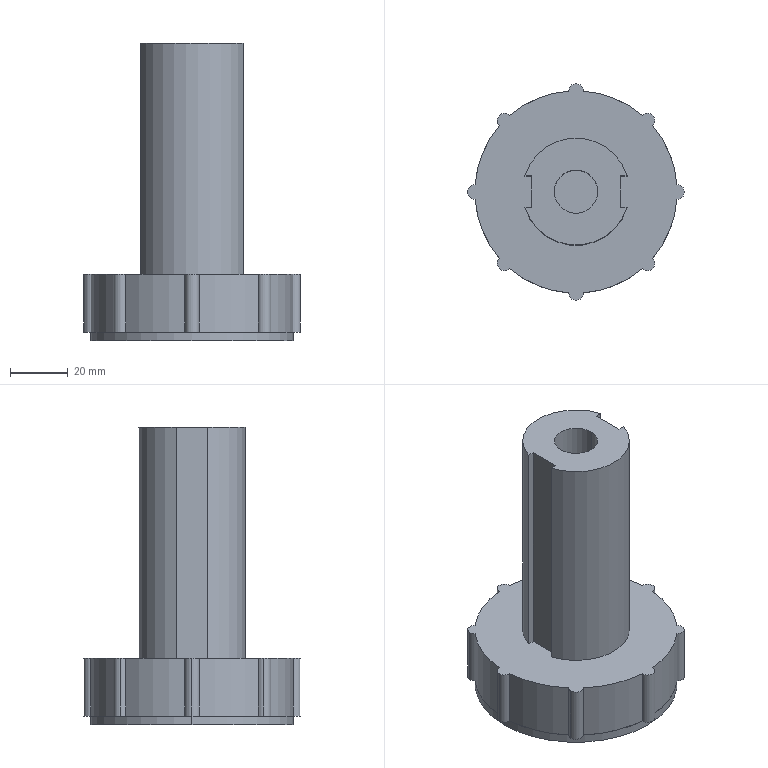Part | SolidWorks | features ICE 4, Extrusion 1, Shell 1 | 2 solids | 43 faces | box 75 x 75 x 103 mm | volume 101976 mm3 | cylinder 31 | plane 12 | commonest cylinder face diameters 5 x15 70 x10 15 x2 37 x2 64 x2
STEP:
#1=CARTESIAN_POINT('',(7.5,0.,17.));
#2=VERTEX_POINT('',#1);
#3=CARTESIAN_POINT('',(-7.5,0.,17.));
#4=VERTEX_POINT('',#3);
#5=CARTESIAN_POINT('',(0.,0.,17.));
#6=DIRECTION('',(0.,0.,-1.));
#7=DIRECTION('',(1.,0.,0.));
#8=AXIS2_PLACEMENT_3D('',#5,#6,#7);
#9=CIRCLE('',#8,7.5);
#10=EDGE_CURVE('',#2,#4,#9,.T.);
#11=ORIENTED_EDGE('',*,*,#10,.T.);
#12=CARTESIAN_POINT('',(-7.5,0.,100.));
#13=VERTEX_POINT('',#12);
#14=CARTESIAN_POINT('',(-7.5,0.,-0.001));
#15=DIRECTION('',(0.,0.,1.));
#16=VECTOR('',#15,1000.);
#17=LINE('',#14,#16);
#18=EDGE_CURVE('',#4,#13,#17,.T.);
#19=ORIENTED_EDGE('',*,*,#18,.T.);
#20=CARTESIAN_POINT('',(7.5,0.,100.));
#21=VERTEX_POINT('',#20);
#22=CARTESIAN_POINT('',(0.,0.,100.));
#23=DIRECTION('',(0.,0.,1.));
#24=DIRECTION('',(1.,0.,0.));
#25=AXIS2_PLACEMENT_3D('',#22,#23,#24);
#26=CIRCLE('',#25,7.5);
#27=EDGE_CURVE('',#13,#21,#26,.T.);
#28=ORIENTED_EDGE('',*,*,#27,.T.);
#29=CARTESIAN_POINT('',(7.5,0.,-0.001));
#30=DIRECTION('',(0.,0.,1.));
#31=VECTOR('',#30,1000.);
#32=LINE('',#29,#31);
#33=EDGE_CURVE('',#2,#21,#32,.T.);
#34=ORIENTED_EDGE('',*,*,#33,.F.);
#35=EDGE_LOOP('',(#11,#19,#28,#34));
#36=FACE_OUTER_BOUND('',#35,.T.);
#37=CARTESIAN_POINT('',(0.,0.,-0.001));
#38=DIRECTION('',(0.,0.,1.));
#39=DIRECTION('',(1.,0.,0.));
#40=AXIS2_PLACEMENT_3D('',#37,#38,#39);
#41=CYLINDRICAL_SURFACE('',#40,7.5);
#42=ADVANCED_FACE('',(#36),#41,.F.);
#43=CARTESIAN_POINT('',(-32.,0.,17.));
#44=VERTEX_POINT('',#43);
#45=CARTESIAN_POINT('',(32.,0.,17.));
#46=VERTEX_POINT('',#45);
#47=CARTESIAN_POINT('',(0.,0.,17.));
#48=DIRECTION('',(0.,0.,1.));
#49=DIRECTION('',(1.,0.,0.));
#50=AXIS2_PLACEMENT_3D('',#47,#48,#49);
#51=CIRCLE('',#50,32.);
#52=EDGE_CURVE('',#44,#46,#51,.T.);
#53=ORIENTED_EDGE('',*,*,#52,.T.);
#54=CARTESIAN_POINT('',(32.,0.,0.));
#55=VERTEX_POINT('',#54);
#56=CARTESIAN_POINT('',(32.,0.,20.));
#57=DIRECTION('',(0.,0.,-1.));
#58=VECTOR('',#57,1000.);
#59=LINE('',#56,#58);
#60=EDGE_CURVE('',#46,#55,#59,.T.);
#61=ORIENTED_EDGE('',*,*,#60,.T.);
#62=CARTESIAN_POINT('',(-32.,0.,0.));
#63=VERTEX_POINT('',#62);
#64=CARTESIAN_POINT('',(0.,0.,0.));
#65=DIRECTION('',(0.,0.,1.));
#66=DIRECTION('',(1.,0.,0.));
#67=AXIS2_PLACEMENT_3D('',#64,#65,#66);
#68=CIRCLE('',#67,32.);
#69=EDGE_CURVE('',#63,#55,#68,.T.);
#70=ORIENTED_EDGE('',*,*,#69,.F.);
#71=CARTESIAN_POINT('',(-32.,0.,20.));
#72=DIRECTION('',(0.,0.,-1.));
#73=VECTOR('',#72,1000.);
#74=LINE('',#71,#73);
#75=EDGE_CURVE('',#44,#63,#74,.T.);
#76=ORIENTED_EDGE('',*,*,#75,.F.);
#77=EDGE_LOOP('',(#53,#61,#70,#76));
#78=FACE_OUTER_BOUND('',#77,.T.);
#79=CARTESIAN_POINT('',(0.,0.,20.));
#80=DIRECTION('',(0.,0.,-1.));
#81=DIRECTION('',(-1.,0.,0.));
#82=AXIS2_PLACEMENT_3D('',#79,#80,#81);
#83=CYLINDRICAL_SURFACE('',#82,32.);
#84=ADVANCED_FACE('',(#78),#83,.F.);
#85=CARTESIAN_POINT('',(2.5,-35.,20.));
#86=VERTEX_POINT('',#85);
#87=CARTESIAN_POINT('',(2.498,-34.911,20.));
#88=VERTEX_POINT('',#87);
#89=CARTESIAN_POINT('',(0.,-35.,20.));
#90=DIRECTION('',(0.,0.,1.));
#91=DIRECTION('',(1.,0.,0.));
#92=AXIS2_PLACEMENT_3D('',#89,#90,#91);
#93=CIRCLE('',#92,2.5);
#94=EDGE_CURVE('',#86,#88,#93,.T.);
#95=ORIENTED_EDGE('',*,*,#94,.F.);
#96=CARTESIAN_POINT('',(2.5,-35.,0.));
#97=VERTEX_POINT('',#96);
#98=CARTESIAN_POINT('',(2.5,-35.,20.));
#99=DIRECTION('',(0.,0.,-1.));
#100=VECTOR('',#99,1000.);
#101=LINE('',#98,#100);
#102=EDGE_CURVE('',#86,#97,#101,.T.);
#103=ORIENTED_EDGE('',*,*,#102,.T.);
#104=CARTESIAN_POINT('',(2.498,-34.911,0.));
#105=VERTEX_POINT('',#104);
#106=CARTESIAN_POINT('',(0.,-35.,0.));
#107=DIRECTION('',(0.,0.,1.));
#108=DIRECTION('',(1.,0.,0.));
#109=AXIS2_PLACEMENT_3D('',#106,#107,#108);
#110=CIRCLE('',#109,2.5);
#111=EDGE_CURVE('',#97,#105,#110,.T.);
#112=ORIENTED_EDGE('',*,*,#111,.T.);
#113=CARTESIAN_POINT('',(2.498,-34.911,20.));
#114=DIRECTION('',(0.,0.,-1.));
#115=VECTOR('',#114,1000.);
#116=LINE('',#113,#115);
#117=EDGE_CURVE('',#88,#105,#116,.T.);
#118=ORIENTED_EDGE('',*,*,#117,.F.);
#119=EDGE_LOOP('',(#95,#103,#112,#118));
#120=FACE_OUTER_BOUND('',#119,.T.);
#121=CARTESIAN_POINT('',(0.,-35.,20.));
#122=DIRECTION('',(0.,0.,-1.));
#123=DIRECTION('',(-1.,0.,0.));
#124=AXIS2_PLACEMENT_3D('',#121,#122,#123);
#125=CYLINDRICAL_SURFACE('',#124,2.5);
#126=ADVANCED_FACE('',(#120),#125,.T.);
#127=ORIENTED_EDGE('',*,*,#102,.F.);
#128=CARTESIAN_POINT('',(-2.5,-35.,20.));
#129=VERTEX_POINT('',#128);
#130=CARTESIAN_POINT('',(0.,-35.,20.));
#131=DIRECTION('',(0.,0.,1.));
#132=DIRECTION('',(1.,0.,0.));
#133=AXIS2_PLACEMENT_3D('',#130,#131,#132);
#134=CIRCLE('',#133,2.5);
#135=EDGE_CURVE('',#129,#86,#134,.T.);
#136=ORIENTED_EDGE('',*,*,#135,.F.);
#137=CARTESIAN_POINT('',(-2.5,-35.,0.));
#138=VERTEX_POINT('',#137);
#139=CARTESIAN_POINT('',(-2.5,-35.,20.));
#140=DIRECTION('',(0.,0.,-1.));
#141=VECTOR('',#140,1000.);
#142=LINE('',#139,#141);
#143=EDGE_CURVE('',#129,#138,#142,.T.);
#144=ORIENTED_EDGE('',*,*,#143,.T.);
#145=CARTESIAN_POINT('',(0.,-35.,0.));
#146=DIRECTION('',(0.,0.,1.));
#147=DIRECTION('',(1.,0.,0.));
#148=AXIS2_PLACEMENT_3D('',#145,#146,#147);
#149=CIRCLE('',#148,2.5);
#150=EDGE_CURVE('',#138,#97,#149,.T.);
#151=ORIENTED_EDGE('',*,*,#150,.T.);
#152=EDGE_LOOP('',(#127,#136,#144,#151));
#153=FACE_OUTER_BOUND('',#152,.T.);
#154=CARTESIAN_POINT('',(0.,-35.,20.));
#155=DIRECTION('',(0.,0.,-1.));
#156=DIRECTION('',(-1.,0.,0.));
#157=AXIS2_PLACEMENT_3D('',#154,#155,#156);
#158=CYLINDRICAL_SURFACE('',#157,2.5);
#159=ADVANCED_FACE('',(#153),#158,.T.);
#160=CARTESIAN_POINT('',(-27.249,-24.749,20.));
#161=VERTEX_POINT('',#160);
#162=CARTESIAN_POINT('',(-22.919,-26.452,20.));
#163=VERTEX_POINT('',#162);
#164=CARTESIAN_POINT('',(-24.749,-24.749,20.));
#165=DIRECTION('',(0.,0.,1.));
#166=DIRECTION('',(1.,0.,0.));
#167=AXIS2_PLACEMENT_3D('',#164,#165,#166);
#168=CIRCLE('',#167,2.5);
#169=EDGE_CURVE('',#161,#163,#168,.T.);
#170=ORIENTED_EDGE('',*,*,#169,.F.);
#171=CARTESIAN_POINT('',(-27.249,-24.749,0.));
#172=VERTEX_POINT('',#171);
#173=CARTESIAN_POINT('',(-27.249,-24.749,20.));
#174=DIRECTION('',(0.,0.,-1.));
#175=VECTOR('',#174,1000.);
#176=LINE('',#173,#175);
#177=EDGE_CURVE('',#161,#172,#176,.T.);
#178=ORIENTED_EDGE('',*,*,#177,.T.);
#179=CARTESIAN_POINT('',(-22.919,-26.452,0.));
#180=VERTEX_POINT('',#179);
#181=CARTESIAN_POINT('',(-24.749,-24.749,0.));
#182=DIRECTION('',(0.,0.,1.));
#183=DIRECTION('',(1.,0.,0.));
#184=AXIS2_PLACEMENT_3D('',#181,#182,#183);
#185=CIRCLE('',#184,2.5);
#186=EDGE_CURVE('',#172,#180,#185,.T.);
#187=ORIENTED_EDGE('',*,*,#186,.T.);
#188=CARTESIAN_POINT('',(-22.919,-26.452,20.));
#189=DIRECTION('',(0.,0.,-1.));
#190=VECTOR('',#189,1000.);
#191=LINE('',#188,#190);
#192=EDGE_CURVE('',#163,#180,#191,.T.);
#193=ORIENTED_EDGE('',*,*,#192,.F.);
#194=EDGE_LOOP('',(#170,#178,#187,#193));
#195=FACE_OUTER_BOUND('',#194,.T.);
#196=CARTESIAN_POINT('',(-24.749,-24.749,20.));
#197=DIRECTION('',(0.,0.,-1.));
#198=DIRECTION('',(-1.,0.,0.));
#199=AXIS2_PLACEMENT_3D('',#196,#197,#198);
#200=CYLINDRICAL_SURFACE('',#199,2.5);
#201=ADVANCED_FACE('',(#195),#200,.T.);
#202=CARTESIAN_POINT('',(-37.5,0.,20.));
#203=VERTEX_POINT('',#202);
#204=CARTESIAN_POINT('',(-34.911,-2.498,20.));
#205=VERTEX_POINT('',#204);
#206=CARTESIAN_POINT('',(-35.,0.,20.));
#207=DIRECTION('',(0.,0.,1.));
#208=DIRECTION('',(1.,0.,0.));
#209=AXIS2_PLACEMENT_3D('',#206,#207,#208);
#210=CIRCLE('',#209,2.5);
#211=EDGE_CURVE('',#203,#205,#210,.T.);
#212=ORIENTED_EDGE('',*,*,#211,.F.);
#213=CARTESIAN_POINT('',(-37.5,0.,0.));
#214=VERTEX_POINT('',#213);
#215=CARTESIAN_POINT('',(-37.5,0.,20.));
#216=DIRECTION('',(0.,0.,-1.));
#217=VECTOR('',#216,1000.);
#218=LINE('',#215,#217);
#219=EDGE_CURVE('',#203,#214,#218,.T.);
#220=ORIENTED_EDGE('',*,*,#219,.T.);
#221=CARTESIAN_POINT('',(-34.911,-2.498,0.));
#222=VERTEX_POINT('',#221);
#223=CARTESIAN_POINT('',(-35.,0.,0.));
#224=DIRECTION('',(0.,0.,1.));
#225=DIRECTION('',(1.,0.,0.));
#226=AXIS2_PLACEMENT_3D('',#223,#224,#225);
#227=CIRCLE('',#226,2.5);
#228=EDGE_CURVE('',#214,#222,#227,.T.);
#229=ORIENTED_EDGE('',*,*,#228,.T.);
#230=CARTESIAN_POINT('',(-34.911,-2.498,20.));
#231=DIRECTION('',(0.,0.,-1.));
#232=VECTOR('',#231,1000.);
#233=LINE('',#230,#232);
#234=EDGE_CURVE('',#205,#222,#233,.T.);
#235=ORIENTED_EDGE('',*,*,#234,.F.);
#236=EDGE_LOOP('',(#212,#220,#229,#235));
#237=FACE_OUTER_BOUND('',#236,.T.);
#238=CARTESIAN_POINT('',(-35.,0.,20.));
#239=DIRECTION('',(0.,0.,-1.));
#240=DIRECTION('',(-1.,0.,0.));
#241=AXIS2_PLACEMENT_3D('',#238,#239,#240);
#242=CYLINDRICAL_SURFACE('',#241,2.5);
#243=ADVANCED_FACE('',(#237),#242,.T.);
#244=CARTESIAN_POINT('',(-27.249,24.749,20.));
#245=VERTEX_POINT('',#244);
#246=CARTESIAN_POINT('',(-26.452,22.919,20.));
#247=VERTEX_POINT('',#246);
#248=CARTESIAN_POINT('',(-24.749,24.749,20.));
#249=DIRECTION('',(0.,0.,1.));
#250=DIRECTION('',(1.,0.,0.));
#251=AXIS2_PLACEMENT_3D('',#248,#249,#250);
#252=CIRCLE('',#251,2.5);
#253=EDGE_CURVE('',#245,#247,#252,.T.);
#254=ORIENTED_EDGE('',*,*,#253,.F.);
#255=CARTESIAN_POINT('',(-27.249,24.749,0.));
#256=VERTEX_POINT('',#255);
#257=CARTESIAN_POINT('',(-27.249,24.749,20.));
#258=DIRECTION('',(0.,0.,-1.));
#259=VECTOR('',#258,1000.);
#260=LINE('',#257,#259);
#261=EDGE_CURVE('',#245,#256,#260,.T.);
#262=ORIENTED_EDGE('',*,*,#261,.T.);
#263=CARTESIAN_POINT('',(-26.452,22.919,0.));
#264=VERTEX_POINT('',#263);
#265=CARTESIAN_POINT('',(-24.749,24.749,0.));
#266=DIRECTION('',(0.,0.,1.));
#267=DIRECTION('',(1.,0.,0.));
#268=AXIS2_PLACEMENT_3D('',#265,#266,#267);
#269=CIRCLE('',#268,2.5);
#270=EDGE_CURVE('',#256,#264,#269,.T.);
#271=ORIENTED_EDGE('',*,*,#270,.T.);
#272=CARTESIAN_POINT('',(-26.452,22.919,20.));
#273=DIRECTION('',(0.,0.,-1.));
#274=VECTOR('',#273,1000.);
#275=LINE('',#272,#274);
#276=EDGE_CURVE('',#247,#264,#275,.T.);
#277=ORIENTED_EDGE('',*,*,#276,.F.);
#278=EDGE_LOOP('',(#254,#262,#271,#277));
#279=FACE_OUTER_BOUND('',#278,.T.);
#280=CARTESIAN_POINT('',(-24.749,24.749,20.));
#281=DIRECTION('',(0.,0.,-1.));
#282=DIRECTION('',(-1.,0.,0.));
#283=AXIS2_PLACEMENT_3D('',#280,#281,#282);
#284=CYLINDRICAL_SURFACE('',#283,2.5);
#285=ADVANCED_FACE('',(#279),#284,.T.);
#286=CARTESIAN_POINT('',(2.5,35.,20.));
#287=VERTEX_POINT('',#286);
#288=CARTESIAN_POINT('',(-2.5,35.,20.));
#289=VERTEX_POINT('',#288);
#290=CARTESIAN_POINT('',(0.,35.,20.));
#291=DIRECTION('',(0.,0.,1.));
#292=DIRECTION('',(1.,0.,0.));
#293=AXIS2_PLACEMENT_3D('',#290,#291,#292);
#294=CIRCLE('',#293,2.5);
#295=EDGE_CURVE('',#287,#289,#294,.T.);
#296=ORIENTED_EDGE('',*,*,#295,.F.);
#297=CARTESIAN_POINT('',(2.5,35.,0.));
#298=VERTEX_POINT('',#297);
#299=CARTESIAN_POINT('',(2.5,35.,20.));
#300=DIRECTION('',(0.,0.,-1.));
#301=VECTOR('',#300,1000.);
#302=LINE('',#299,#301);
#303=EDGE_CURVE('',#287,#298,#302,.T.);
#304=ORIENTED_EDGE('',*,*,#303,.T.);
#305=CARTESIAN_POINT('',(-2.5,35.,0.));
#306=VERTEX_POINT('',#305);
#307=CARTESIAN_POINT('',(0.,35.,0.));
#308=DIRECTION('',(0.,0.,1.));
#309=DIRECTION('',(1.,0.,0.));
#310=AXIS2_PLACEMENT_3D('',#307,#308,#309);
#311=CIRCLE('',#310,2.5);
#312=EDGE_CURVE('',#298,#306,#311,.T.);
#313=ORIENTED_EDGE('',*,*,#312,.T.);
#314=CARTESIAN_POINT('',(-2.5,35.,20.));
#315=DIRECTION('',(0.,0.,-1.));
#316=VECTOR('',#315,1000.);
#317=LINE('',#314,#316);
#318=EDGE_CURVE('',#289,#306,#317,.T.);
#319=ORIENTED_EDGE('',*,*,#318,.F.);
#320=EDGE_LOOP('',(#296,#304,#313,#319));
#321=FACE_OUTER_BOUND('',#320,.T.);
#322=CARTESIAN_POINT('',(0.,35.,20.));
#323=DIRECTION('',(0.,0.,-1.));
#324=DIRECTION('',(-1.,0.,0.));
#325=AXIS2_PLACEMENT_3D('',#322,#323,#324);
#326=CYLINDRICAL_SURFACE('',#325,2.5);
#327=ADVANCED_FACE('',(#321),#326,.T.);
#328=CARTESIAN_POINT('',(-2.498,34.911,20.));
#329=VERTEX_POINT('',#328);
#330=CARTESIAN_POINT('',(0.,35.,20.));
#331=DIRECTION('',(0.,0.,1.));
#332=DIRECTION('',(1.,0.,0.));
#333=AXIS2_PLACEMENT_3D('',#330,#331,#332);
#334=CIRCLE('',#333,2.5);
#335=EDGE_CURVE('',#289,#329,#334,.T.);
#336=ORIENTED_EDGE('',*,*,#335,.F.);
#337=ORIENTED_EDGE('',*,*,#318,.T.);
#338=CARTESIAN_POINT('',(-2.498,34.911,0.));
#339=VERTEX_POINT('',#338);
#340=CARTESIAN_POINT('',(0.,35.,0.));
#341=DIRECTION('',(0.,0.,1.));
#342=DIRECTION('',(1.,0.,0.));
#343=AXIS2_PLACEMENT_3D('',#340,#341,#342);
#344=CIRCLE('',#343,2.5);
#345=EDGE_CURVE('',#306,#339,#344,.T.);
#346=ORIENTED_EDGE('',*,*,#345,.T.);
#347=CARTESIAN_POINT('',(-2.498,34.911,20.));
#348=DIRECTION('',(0.,0.,-1.));
#349=VECTOR('',#348,1000.);
#350=LINE('',#347,#349);
#351=EDGE_CURVE('',#329,#339,#350,.T.);
#352=ORIENTED_EDGE('',*,*,#351,.F.);
#353=EDGE_LOOP('',(#336,#337,#346,#352));
#354=FACE_OUTER_BOUND('',#353,.T.);
#355=CARTESIAN_POINT('',(0.,35.,20.));
#356=DIRECTION('',(0.,0.,-1.));
#357=DIRECTION('',(-1.,0.,0.));
#358=AXIS2_PLACEMENT_3D('',#355,#356,#357);
#359=CYLINDRICAL_SURFACE('',#358,2.5);
#360=ADVANCED_FACE('',(#354),#359,.T.);
#361=CARTESIAN_POINT('',(-17.664,-5.5,20.));
#362=VERTEX_POINT('',#361);
#363=CARTESIAN_POINT('',(17.664,-5.5,20.));
#364=VERTEX_POINT('',#363);
#365=CARTESIAN_POINT('',(0.,0.,20.));
#366=DIRECTION('',(0.,0.,1.));
#367=DIRECTION('',(1.,0.,0.));
#368=AXIS2_PLACEMENT_3D('',#365,#366,#367);
#369=CIRCLE('',#368,18.5);
#370=EDGE_CURVE('',#362,#364,#369,.T.);
#371=ORIENTED_EDGE('',*,*,#370,.T.);
#372=CARTESIAN_POINT('',(17.664,-5.5,100.));
#373=VERTEX_POINT('',#372);
#374=CARTESIAN_POINT('',(17.664,-5.5,8.598));
#375=DIRECTION('',(0.,0.,1.));
#376=VECTOR('',#375,1000.);
#377=LINE('',#374,#376);
#378=EDGE_CURVE('',#364,#373,#377,.T.);
#379=ORIENTED_EDGE('',*,*,#378,.T.);
#380=CARTESIAN_POINT('',(-17.664,-5.5,100.));
#381=VERTEX_POINT('',#380);
#382=CARTESIAN_POINT('',(0.,0.,100.));
#383=DIRECTION('',(0.,0.,1.));
#384=DIRECTION('',(1.,0.,0.));
#385=AXIS2_PLACEMENT_3D('',#382,#383,#384);
#386=CIRCLE('',#385,18.5);
#387=EDGE_CURVE('',#381,#373,#386,.T.);
#388=ORIENTED_EDGE('',*,*,#387,.F.);
#389=CARTESIAN_POINT('',(-17.664,-5.5,8.598));
#390=DIRECTION('',(0.,0.,1.));
#391=VECTOR('',#390,1000.);
#392=LINE('',#389,#391);
#393=EDGE_CURVE('',#362,#381,#392,.T.);
#394=ORIENTED_EDGE('',*,*,#393,.F.);
#395=EDGE_LOOP('',(#371,#379,#388,#394));
#396=FACE_OUTER_BOUND('',#395,.T.);
#397=CARTESIAN_POINT('',(0.,0.,100.));
#398=DIRECTION('',(0.,0.,-1.));
#399=DIRECTION('',(-1.,0.,0.));
#400=AXIS2_PLACEMENT_3D('',#397,#398,#399);
#401=CYLINDRICAL_SURFACE('',#400,18.5);
#402=ADVANCED_FACE('',(#396),#401,.T.);
#403=CARTESIAN_POINT('',(22.919,-26.452,20.));
#404=VERTEX_POINT('',#403);
#405=CARTESIAN_POINT('',(0.,0.,20.));
#406=DIRECTION('',(0.,0.,1.));
#407=DIRECTION('',(1.,0.,0.));
#408=AXIS2_PLACEMENT_3D('',#405,#406,#407);
#409=CIRCLE('',#408,35.);
#410=EDGE_CURVE('',#88,#404,#409,.T.);
#411=ORIENTED_EDGE('',*,*,#410,.T.);
#412=CARTESIAN_POINT('',(26.452,-22.919,20.));
#413=VERTEX_POINT('',#412);
#414=CARTESIAN_POINT('',(24.749,-24.749,20.));
#415=DIRECTION('',(0.,0.,1.));
#416=DIRECTION('',(1.,0.,0.));
#417=AXIS2_PLACEMENT_3D('',#414,#415,#416);
#418=CIRCLE('',#417,2.5);
#419=EDGE_CURVE('',#404,#413,#418,.T.);
#420=ORIENTED_EDGE('',*,*,#419,.T.);
#421=CARTESIAN_POINT('',(34.911,-2.498,20.));
#422=VERTEX_POINT('',#421);
#423=CARTESIAN_POINT('',(0.,0.,20.));
#424=DIRECTION('',(0.,0.,1.));
#425=DIRECTION('',(1.,0.,0.));
#426=AXIS2_PLACEMENT_3D('',#423,#424,#425);
#427=CIRCLE('',#426,35.);
#428=EDGE_CURVE('',#413,#422,#427,.T.);
#429=ORIENTED_EDGE('',*,*,#428,.T.);
#430=CARTESIAN_POINT('',(34.911,2.498,20.));
#431=VERTEX_POINT('',#430);
#432=CARTESIAN_POINT('',(35.,0.,20.));
#433=DIRECTION('',(0.,0.,1.));
#434=DIRECTION('',(1.,0.,0.));
#435=AXIS2_PLACEMENT_3D('',#432,#433,#434);
#436=CIRCLE('',#435,2.5);
#437=EDGE_CURVE('',#422,#431,#436,.T.);
#438=ORIENTED_EDGE('',*,*,#437,.T.);
#439=CARTESIAN_POINT('',(26.452,22.919,20.));
#440=VERTEX_POINT('',#439);
#441=CARTESIAN_POINT('',(0.,0.,20.));
#442=DIRECTION('',(0.,0.,1.));
#443=DIRECTION('',(1.,0.,0.));
#444=AXIS2_PLACEMENT_3D('',#441,#442,#443);
#445=CIRCLE('',#444,35.);
#446=EDGE_CURVE('',#431,#440,#445,.T.);
#447=ORIENTED_EDGE('',*,*,#446,.T.);
#448=CARTESIAN_POINT('',(22.919,26.452,20.));
#449=VERTEX_POINT('',#448);
#450=CARTESIAN_POINT('',(24.749,24.749,20.));
#451=DIRECTION('',(0.,0.,1.));
#452=DIRECTION('',(1.,0.,0.));
#453=AXIS2_PLACEMENT_3D('',#450,#451,#452);
#454=CIRCLE('',#453,2.5);
#455=EDGE_CURVE('',#440,#449,#454,.T.);
#456=ORIENTED_EDGE('',*,*,#455,.T.);
#457=CARTESIAN_POINT('',(2.498,34.911,20.));
#458=VERTEX_POINT('',#457);
#459=CARTESIAN_POINT('',(0.,0.,20.));
#460=DIRECTION('',(0.,0.,1.));
#461=DIRECTION('',(1.,0.,0.));
#462=AXIS2_PLACEMENT_3D('',#459,#460,#461);
#463=CIRCLE('',#462,35.);
#464=EDGE_CURVE('',#449,#458,#463,.T.);
#465=ORIENTED_EDGE('',*,*,#464,.T.);
#466=CARTESIAN_POINT('',(0.,35.,20.));
#467=DIRECTION('',(0.,0.,1.));
#468=DIRECTION('',(1.,0.,0.));
#469=AXIS2_PLACEMENT_3D('',#466,#467,#468);
#470=CIRCLE('',#469,2.5);
#471=EDGE_CURVE('',#458,#287,#470,.T.);
#472=ORIENTED_EDGE('',*,*,#471,.T.);
#473=ORIENTED_EDGE('',*,*,#295,.T.);
#474=ORIENTED_EDGE('',*,*,#335,.T.);
#475=CARTESIAN_POINT('',(-22.919,26.452,20.));
#476=VERTEX_POINT('',#475);
#477=CARTESIAN_POINT('',(0.,0.,20.));
#478=DIRECTION('',(0.,0.,1.));
#479=DIRECTION('',(1.,0.,0.));
#480=AXIS2_PLACEMENT_3D('',#477,#478,#479);
#481=CIRCLE('',#480,35.);
#482=EDGE_CURVE('',#329,#476,#481,.T.);
#483=ORIENTED_EDGE('',*,*,#482,.T.);
#484=CARTESIAN_POINT('',(-24.749,24.749,20.));
#485=DIRECTION('',(0.,0.,1.));
#486=DIRECTION('',(1.,0.,0.));
#487=AXIS2_PLACEMENT_3D('',#484,#485,#486);
#488=CIRCLE('',#487,2.5);
#489=EDGE_CURVE('',#476,#245,#488,.T.);
#490=ORIENTED_EDGE('',*,*,#489,.T.);
#491=ORIENTED_EDGE('',*,*,#253,.T.);
#492=CARTESIAN_POINT('',(-34.911,2.498,20.));
#493=VERTEX_POINT('',#492);
#494=CARTESIAN_POINT('',(0.,0.,20.));
#495=DIRECTION('',(0.,0.,1.));
#496=DIRECTION('',(1.,0.,0.));
#497=AXIS2_PLACEMENT_3D('',#494,#495,#496);
#498=CIRCLE('',#497,35.);
#499=EDGE_CURVE('',#247,#493,#498,.T.);
#500=ORIENTED_EDGE('',*,*,#499,.T.);
#501=CARTESIAN_POINT('',(-35.,0.,20.));
#502=DIRECTION('',(0.,0.,1.));
#503=DIRECTION('',(1.,0.,0.));
#504=AXIS2_PLACEMENT_3D('',#501,#502,#503);
#505=CIRCLE('',#504,2.5);
#506=EDGE_CURVE('',#493,#203,#505,.T.);
#507=ORIENTED_EDGE('',*,*,#506,.T.);
#508=ORIENTED_EDGE('',*,*,#211,.T.);
#509=CARTESIAN_POINT('',(-26.452,-22.919,20.));
#510=VERTEX_POINT('',#509);
#511=CARTESIAN_POINT('',(0.,0.,20.));
#512=DIRECTION('',(0.,0.,1.));
#513=DIRECTION('',(1.,0.,0.));
#514=AXIS2_PLACEMENT_3D('',#511,#512,#513);
#515=CIRCLE('',#514,35.);
#516=EDGE_CURVE('',#205,#510,#515,.T.);
#517=ORIENTED_EDGE('',*,*,#516,.T.);
#518=CARTESIAN_POINT('',(-24.749,-24.749,20.));
#519=DIRECTION('',(0.,0.,1.));
#520=DIRECTION('',(1.,0.,0.));
#521=AXIS2_PLACEMENT_3D('',#518,#519,#520);
#522=CIRCLE('',#521,2.5);
#523=EDGE_CURVE('',#510,#161,#522,.T.);
#524=ORIENTED_EDGE('',*,*,#523,.T.);
#525=ORIENTED_EDGE('',*,*,#169,.T.);
#526=CARTESIAN_POINT('',(-2.498,-34.911,20.));
#527=VERTEX_POINT('',#526);
#528=CARTESIAN_POINT('',(0.,0.,20.));
#529=DIRECTION('',(0.,0.,1.));
#530=DIRECTION('',(1.,0.,0.));
#531=AXIS2_PLACEMENT_3D('',#528,#529,#530);
#532=CIRCLE('',#531,35.);
#533=EDGE_CURVE('',#163,#527,#532,.T.);
#534=ORIENTED_EDGE('',*,*,#533,.T.);
#535=CARTESIAN_POINT('',(0.,-35.,20.));
#536=DIRECTION('',(0.,0.,1.));
#537=DIRECTION('',(1.,0.,0.));
#538=AXIS2_PLACEMENT_3D('',#535,#536,#537);
#539=CIRCLE('',#538,2.5);
#540=EDGE_CURVE('',#527,#129,#539,.T.);
#541=ORIENTED_EDGE('',*,*,#540,.T.);
#542=ORIENTED_EDGE('',*,*,#135,.T.);
#543=ORIENTED_EDGE('',*,*,#94,.T.);
#544=EDGE_LOOP('',(#411,#420,#429,#438,#447,#456,#465,#472,#473,#474,#483,#490,#491,#500,#507,#508,#517,#524,#525,#534,#541,#542,#543));
#545=FACE_OUTER_BOUND('',#544,.T.);
#546=ORIENTED_EDGE('',*,*,#370,.F.);
#547=CARTESIAN_POINT('',(-15.5,-5.5,20.));
#548=VERTEX_POINT('',#547);
#549=CARTESIAN_POINT('',(-17.664,-5.5,20.));
#550=DIRECTION('',(-1.,0.,0.));
#551=VECTOR('',#550,1000.);
#552=LINE('',#549,#551);
#553=EDGE_CURVE('',#548,#362,#552,.T.);
#554=ORIENTED_EDGE('',*,*,#553,.F.);
#555=CARTESIAN_POINT('',(-15.5,5.5,20.));
#556=VERTEX_POINT('',#555);
#557=CARTESIAN_POINT('',(-15.5,5.5,20.));
#558=DIRECTION('',(0.,-1.,0.));
#559=VECTOR('',#558,1000.);
#560=LINE('',#557,#559);
#561=EDGE_CURVE('',#556,#548,#560,.T.);
#562=ORIENTED_EDGE('',*,*,#561,.F.);
#563=CARTESIAN_POINT('',(-17.664,5.5,20.));
#564=VERTEX_POINT('',#563);
#565=CARTESIAN_POINT('',(-17.664,5.5,20.));
#566=DIRECTION('',(1.,0.,0.));
#567=VECTOR('',#566,1000.);
#568=LINE('',#565,#567);
#569=EDGE_CURVE('',#564,#556,#568,.T.);
#570=ORIENTED_EDGE('',*,*,#569,.F.);
#571=CARTESIAN_POINT('',(17.664,5.5,20.));
#572=VERTEX_POINT('',#571);
#573=CARTESIAN_POINT('',(0.,0.,20.));
#574=DIRECTION('',(0.,0.,1.));
#575=DIRECTION('',(1.,0.,0.));
#576=AXIS2_PLACEMENT_3D('',#573,#574,#575);
#577=CIRCLE('',#576,18.5);
#578=EDGE_CURVE('',#572,#564,#577,.T.);
#579=ORIENTED_EDGE('',*,*,#578,.F.);
#580=CARTESIAN_POINT('',(15.5,5.5,20.));
#581=VERTEX_POINT('',#580);
#582=CARTESIAN_POINT('',(17.664,5.5,20.));
#583=DIRECTION('',(1.,0.,0.));
#584=VECTOR('',#583,1000.);
#585=LINE('',#582,#584);
#586=EDGE_CURVE('',#581,#572,#585,.T.);
#587=ORIENTED_EDGE('',*,*,#586,.F.);
#588=CARTESIAN_POINT('',(15.5,-5.5,20.));
#589=VERTEX_POINT('',#588);
#590=CARTESIAN_POINT('',(15.5,5.5,20.));
#591=DIRECTION('',(0.,1.,0.));
#592=VECTOR('',#591,1000.);
#593=LINE('',#590,#592);
#594=EDGE_CURVE('',#589,#581,#593,.T.);
#595=ORIENTED_EDGE('',*,*,#594,.F.);
#596=CARTESIAN_POINT('',(17.664,-5.5,20.));
#597=DIRECTION('',(-1.,0.,0.));
#598=VECTOR('',#597,1000.);
#599=LINE('',#596,#598);
#600=EDGE_CURVE('',#364,#589,#599,.T.);
#601=ORIENTED_EDGE('',*,*,#600,.F.);
#602=EDGE_LOOP('',(#546,#554,#562,#570,#579,#587,#595,#601));
#603=FACE_BOUND('',#602,.T.);
#604=CARTESIAN_POINT('',(12.374,-12.374,20.));
#605=DIRECTION('',(0.,0.,1.));
#606=DIRECTION('',(1.,0.,0.));
#607=AXIS2_PLACEMENT_3D('',#604,#605,#606);
#608=PLANE('',#607);
#609=ADVANCED_FACE('',(#545,#603),#608,.T.);
#610=CARTESIAN_POINT('',(22.919,-26.452,0.));
#611=VERTEX_POINT('',#610);
#612=CARTESIAN_POINT('',(0.,0.,0.));
#613=DIRECTION('',(0.,0.,1.));
#614=DIRECTION('',(1.,0.,0.));
#615=AXIS2_PLACEMENT_3D('',#612,#613,#614);
#616=CIRCLE('',#615,35.);
#617=EDGE_CURVE('',#105,#611,#616,.T.);
#618=ORIENTED_EDGE('',*,*,#617,.T.);
#619=CARTESIAN_POINT('',(22.919,-26.452,20.));
#620=DIRECTION('',(0.,0.,-1.));
#621=VECTOR('',#620,1000.);
#622=LINE('',#619,#621);
#623=EDGE_CURVE('',#404,#611,#622,.T.);
#624=ORIENTED_EDGE('',*,*,#623,.F.);
#625=ORIENTED_EDGE('',*,*,#410,.F.);
#626=ORIENTED_EDGE('',*,*,#117,.T.);
#627=EDGE_LOOP('',(#618,#624,#625,#626));
#628=FACE_OUTER_BOUND('',#627,.T.);
#629=CARTESIAN_POINT('',(0.,0.,20.));
#630=DIRECTION('',(0.,0.,-1.));
#631=DIRECTION('',(-1.,0.,0.));
#632=AXIS2_PLACEMENT_3D('',#629,#630,#631);
#633=CYLINDRICAL_SURFACE('',#632,35.);
#634=ADVANCED_FACE('',(#628),#633,.T.);
#635=CARTESIAN_POINT('',(26.452,-22.919,0.));
#636=VERTEX_POINT('',#635);
#637=CARTESIAN_POINT('',(24.749,-24.749,0.));
#638=DIRECTION('',(0.,0.,1.));
#639=DIRECTION('',(1.,0.,0.));
#640=AXIS2_PLACEMENT_3D('',#637,#638,#639);
#641=CIRCLE('',#640,2.5);
#642=EDGE_CURVE('',#611,#636,#641,.T.);
#643=ORIENTED_EDGE('',*,*,#642,.T.);
#644=CARTESIAN_POINT('',(26.452,-22.919,20.));
#645=DIRECTION('',(0.,0.,-1.));
#646=VECTOR('',#645,1000.);
#647=LINE('',#644,#646);
#648=EDGE_CURVE('',#413,#636,#647,.T.);
#649=ORIENTED_EDGE('',*,*,#648,.F.);
#650=ORIENTED_EDGE('',*,*,#419,.F.);
#651=ORIENTED_EDGE('',*,*,#623,.T.);
#652=EDGE_LOOP('',(#643,#649,#650,#651));
#653=FACE_OUTER_BOUND('',#652,.T.);
#654=CARTESIAN_POINT('',(24.749,-24.749,20.));
#655=DIRECTION('',(0.,0.,-1.));
#656=DIRECTION('',(-1.,0.,0.));
#657=AXIS2_PLACEMENT_3D('',#654,#655,#656);
#658=CYLINDRICAL_SURFACE('',#657,2.5);
#659=ADVANCED_FACE('',(#653),#658,.T.);
#660=CARTESIAN_POINT('',(34.911,-2.498,0.));
#661=VERTEX_POINT('',#660);
#662=CARTESIAN_POINT('',(0.,0.,0.));
#663=DIRECTION('',(0.,0.,1.));
#664=DIRECTION('',(1.,0.,0.));
#665=AXIS2_PLACEMENT_3D('',#662,#663,#664);
#666=CIRCLE('',#665,35.);
#667=EDGE_CURVE('',#636,#661,#666,.T.);
#668=ORIENTED_EDGE('',*,*,#667,.T.);
#669=CARTESIAN_POINT('',(34.911,-2.498,20.));
#670=DIRECTION('',(0.,0.,-1.));
#671=VECTOR('',#670,1000.);
#672=LINE('',#669,#671);
#673=EDGE_CURVE('',#422,#661,#672,.T.);
#674=ORIENTED_EDGE('',*,*,#673,.F.);
#675=ORIENTED_EDGE('',*,*,#428,.F.);
#676=ORIENTED_EDGE('',*,*,#648,.T.);
#677=EDGE_LOOP('',(#668,#674,#675,#676));
#678=FACE_OUTER_BOUND('',#677,.T.);
#679=CARTESIAN_POINT('',(0.,0.,20.));
#680=DIRECTION('',(0.,0.,-1.));
#681=DIRECTION('',(-1.,0.,0.));
#682=AXIS2_PLACEMENT_3D('',#679,#680,#681);
#683=CYLINDRICAL_SURFACE('',#682,35.);
#684=ADVANCED_FACE('',(#678),#683,.T.);
#685=CARTESIAN_POINT('',(34.911,2.498,0.));
#686=VERTEX_POINT('',#685);
#687=CARTESIAN_POINT('',(35.,0.,0.));
#688=DIRECTION('',(0.,0.,1.));
#689=DIRECTION('',(1.,0.,0.));
#690=AXIS2_PLACEMENT_3D('',#687,#688,#689);
#691=CIRCLE('',#690,2.5);
#692=EDGE_CURVE('',#661,#686,#691,.T.);
#693=ORIENTED_EDGE('',*,*,#692,.T.);
#694=CARTESIAN_POINT('',(34.911,2.498,20.));
#695=DIRECTION('',(0.,0.,-1.));
#696=VECTOR('',#695,1000.);
#697=LINE('',#694,#696);
#698=EDGE_CURVE('',#431,#686,#697,.T.);
#699=ORIENTED_EDGE('',*,*,#698,.F.);
#700=ORIENTED_EDGE('',*,*,#437,.F.);
#701=ORIENTED_EDGE('',*,*,#673,.T.);
#702=EDGE_LOOP('',(#693,#699,#700,#701));
#703=FACE_OUTER_BOUND('',#702,.T.);
#704=CARTESIAN_POINT('',(35.,0.,20.));
#705=DIRECTION('',(0.,0.,-1.));
#706=DIRECTION('',(-1.,0.,0.));
#707=AXIS2_PLACEMENT_3D('',#704,#705,#706);
#708=CYLINDRICAL_SURFACE('',#707,2.5);
#709=ADVANCED_FACE('',(#703),#708,.T.);
#710=CARTESIAN_POINT('',(26.452,22.919,0.));
#711=VERTEX_POINT('',#710);
#712=CARTESIAN_POINT('',(0.,0.,0.));
#713=DIRECTION('',(0.,0.,1.));
#714=DIRECTION('',(1.,0.,0.));
#715=AXIS2_PLACEMENT_3D('',#712,#713,#714);
#716=CIRCLE('',#715,35.);
#717=EDGE_CURVE('',#686,#711,#716,.T.);
#718=ORIENTED_EDGE('',*,*,#717,.T.);
#719=CARTESIAN_POINT('',(26.452,22.919,20.));
#720=DIRECTION('',(0.,0.,-1.));
#721=VECTOR('',#720,1000.);
#722=LINE('',#719,#721);
#723=EDGE_CURVE('',#440,#711,#722,.T.);
#724=ORIENTED_EDGE('',*,*,#723,.F.);
#725=ORIENTED_EDGE('',*,*,#446,.F.);
#726=ORIENTED_EDGE('',*,*,#698,.T.);
#727=EDGE_LOOP('',(#718,#724,#725,#726));
#728=FACE_OUTER_BOUND('',#727,.T.);
#729=CARTESIAN_POINT('',(0.,0.,20.));
#730=DIRECTION('',(0.,0.,-1.));
#731=DIRECTION('',(-1.,0.,0.));
#732=AXIS2_PLACEMENT_3D('',#729,#730,#731);
#733=CYLINDRICAL_SURFACE('',#732,35.);
#734=ADVANCED_FACE('',(#728),#733,.T.);
#735=CARTESIAN_POINT('',(22.919,26.452,0.));
#736=VERTEX_POINT('',#735);
#737=CARTESIAN_POINT('',(24.749,24.749,0.));
#738=DIRECTION('',(0.,0.,1.));
#739=DIRECTION('',(1.,0.,0.));
#740=AXIS2_PLACEMENT_3D('',#737,#738,#739);
#741=CIRCLE('',#740,2.5);
#742=EDGE_CURVE('',#711,#736,#741,.T.);
#743=ORIENTED_EDGE('',*,*,#742,.T.);
#744=CARTESIAN_POINT('',(22.919,26.452,20.));
#745=DIRECTION('',(0.,0.,-1.));
#746=VECTOR('',#745,1000.);
#747=LINE('',#744,#746);
#748=EDGE_CURVE('',#449,#736,#747,.T.);
#749=ORIENTED_EDGE('',*,*,#748,.F.);
#750=ORIENTED_EDGE('',*,*,#455,.F.);
#751=ORIENTED_EDGE('',*,*,#723,.T.);
#752=EDGE_LOOP('',(#743,#749,#750,#751));
#753=FACE_OUTER_BOUND('',#752,.T.);
#754=CARTESIAN_POINT('',(24.749,24.749,20.));
#755=DIRECTION('',(0.,0.,-1.));
#756=DIRECTION('',(-1.,0.,0.));
#757=AXIS2_PLACEMENT_3D('',#754,#755,#756);
#758=CYLINDRICAL_SURFACE('',#757,2.5);
#759=ADVANCED_FACE('',(#753),#758,.T.);
#760=CARTESIAN_POINT('',(2.498,34.911,0.));
#761=VERTEX_POINT('',#760);
#762=CARTESIAN_POINT('',(0.,0.,0.));
#763=DIRECTION('',(0.,0.,1.));
#764=DIRECTION('',(1.,0.,0.));
#765=AXIS2_PLACEMENT_3D('',#762,#763,#764);
#766=CIRCLE('',#765,35.);
#767=EDGE_CURVE('',#736,#761,#766,.T.);
#768=ORIENTED_EDGE('',*,*,#767,.T.);
#769=CARTESIAN_POINT('',(2.498,34.911,20.));
#770=DIRECTION('',(0.,0.,-1.));
#771=VECTOR('',#770,1000.);
#772=LINE('',#769,#771);
#773=EDGE_CURVE('',#458,#761,#772,.T.);
#774=ORIENTED_EDGE('',*,*,#773,.F.);
#775=ORIENTED_EDGE('',*,*,#464,.F.);
#776=ORIENTED_EDGE('',*,*,#748,.T.);
#777=EDGE_LOOP('',(#768,#774,#775,#776));
#778=FACE_OUTER_BOUND('',#777,.T.);
#779=CARTESIAN_POINT('',(0.,0.,20.));
#780=DIRECTION('',(0.,0.,-1.));
#781=DIRECTION('',(-1.,0.,0.));
#782=AXIS2_PLACEMENT_3D('',#779,#780,#781);
#783=CYLINDRICAL_SURFACE('',#782,35.);
#784=ADVANCED_FACE('',(#778),#783,.T.);
#785=ORIENTED_EDGE('',*,*,#303,.F.);
#786=ORIENTED_EDGE('',*,*,#471,.F.);
#787=ORIENTED_EDGE('',*,*,#773,.T.);
#788=CARTESIAN_POINT('',(0.,35.,0.));
#789=DIRECTION('',(0.,0.,1.));
#790=DIRECTION('',(1.,0.,0.));
#791=AXIS2_PLACEMENT_3D('',#788,#789,#790);
#792=CIRCLE('',#791,2.5);
#793=EDGE_CURVE('',#761,#298,#792,.T.);
#794=ORIENTED_EDGE('',*,*,#793,.T.);
#795=EDGE_LOOP('',(#785,#786,#787,#794));
#796=FACE_OUTER_BOUND('',#795,.T.);
#797=CARTESIAN_POINT('',(0.,35.,20.));
#798=DIRECTION('',(0.,0.,-1.));
#799=DIRECTION('',(-1.,0.,0.));
#800=AXIS2_PLACEMENT_3D('',#797,#798,#799);
#801=CYLINDRICAL_SURFACE('',#800,2.5);
#802=ADVANCED_FACE('',(#796),#801,.T.);
#803=CARTESIAN_POINT('',(-22.919,26.452,0.));
#804=VERTEX_POINT('',#803);
#805=CARTESIAN_POINT('',(0.,0.,0.));
#806=DIRECTION('',(0.,0.,1.));
#807=DIRECTION('',(1.,0.,0.));
#808=AXIS2_PLACEMENT_3D('',#805,#806,#807);
#809=CIRCLE('',#808,35.);
#810=EDGE_CURVE('',#339,#804,#809,.T.);
#811=ORIENTED_EDGE('',*,*,#810,.T.);
#812=CARTESIAN_POINT('',(-22.919,26.452,20.));
#813=DIRECTION('',(0.,0.,-1.));
#814=VECTOR('',#813,1000.);
#815=LINE('',#812,#814);
#816=EDGE_CURVE('',#476,#804,#815,.T.);
#817=ORIENTED_EDGE('',*,*,#816,.F.);
#818=ORIENTED_EDGE('',*,*,#482,.F.);
#819=ORIENTED_EDGE('',*,*,#351,.T.);
#820=EDGE_LOOP('',(#811,#817,#818,#819));
#821=FACE_OUTER_BOUND('',#820,.T.);
#822=CARTESIAN_POINT('',(0.,0.,20.));
#823=DIRECTION('',(0.,0.,-1.));
#824=DIRECTION('',(-1.,0.,0.));
#825=AXIS2_PLACEMENT_3D('',#822,#823,#824);
#826=CYLINDRICAL_SURFACE('',#825,35.);
#827=ADVANCED_FACE('',(#821),#826,.T.);
#828=ORIENTED_EDGE('',*,*,#261,.F.);
#829=ORIENTED_EDGE('',*,*,#489,.F.);
#830=ORIENTED_EDGE('',*,*,#816,.T.);
#831=CARTESIAN_POINT('',(-24.749,24.749,0.));
#832=DIRECTION('',(0.,0.,1.));
#833=DIRECTION('',(1.,0.,0.));
#834=AXIS2_PLACEMENT_3D('',#831,#832,#833);
#835=CIRCLE('',#834,2.5);
#836=EDGE_CURVE('',#804,#256,#835,.T.);
#837=ORIENTED_EDGE('',*,*,#836,.T.);
#838=EDGE_LOOP('',(#828,#829,#830,#837));
#839=FACE_OUTER_BOUND('',#838,.T.);
#840=CARTESIAN_POINT('',(-24.749,24.749,20.));
#841=DIRECTION('',(0.,0.,-1.));
#842=DIRECTION('',(-1.,0.,0.));
#843=AXIS2_PLACEMENT_3D('',#840,#841,#842);
#844=CYLINDRICAL_SURFACE('',#843,2.5);
#845=ADVANCED_FACE('',(#839),#844,.T.);
#846=CARTESIAN_POINT('',(-34.911,2.498,0.));
#847=VERTEX_POINT('',#846);
#848=CARTESIAN_POINT('',(0.,0.,0.));
#849=DIRECTION('',(0.,0.,1.));
#850=DIRECTION('',(1.,0.,0.));
#851=AXIS2_PLACEMENT_3D('',#848,#849,#850);
#852=CIRCLE('',#851,35.);
#853=EDGE_CURVE('',#264,#847,#852,.T.);
#854=ORIENTED_EDGE('',*,*,#853,.T.);
#855=CARTESIAN_POINT('',(-34.911,2.498,20.));
#856=DIRECTION('',(0.,0.,-1.));
#857=VECTOR('',#856,1000.);
#858=LINE('',#855,#857);
#859=EDGE_CURVE('',#493,#847,#858,.T.);
#860=ORIENTED_EDGE('',*,*,#859,.F.);
#861=ORIENTED_EDGE('',*,*,#499,.F.);
#862=ORIENTED_EDGE('',*,*,#276,.T.);
#863=EDGE_LOOP('',(#854,#860,#861,#862));
#864=FACE_OUTER_BOUND('',#863,.T.);
#865=CARTESIAN_POINT('',(0.,0.,20.));
#866=DIRECTION('',(0.,0.,-1.));
#867=DIRECTION('',(-1.,0.,0.));
#868=AXIS2_PLACEMENT_3D('',#865,#866,#867);
#869=CYLINDRICAL_SURFACE('',#868,35.);
#870=ADVANCED_FACE('',(#864),#869,.T.);
#871=ORIENTED_EDGE('',*,*,#219,.F.);
#872=ORIENTED_EDGE('',*,*,#506,.F.);
#873=ORIENTED_EDGE('',*,*,#859,.T.);
#874=CARTESIAN_POINT('',(-35.,0.,0.));
#875=DIRECTION('',(0.,0.,1.));
#876=DIRECTION('',(1.,0.,0.));
#877=AXIS2_PLACEMENT_3D('',#874,#875,#876);
#878=CIRCLE('',#877,2.5);
#879=EDGE_CURVE('',#847,#214,#878,.T.);
#880=ORIENTED_EDGE('',*,*,#879,.T.);
#881=EDGE_LOOP('',(#871,#872,#873,#880));
#882=FACE_OUTER_BOUND('',#881,.T.);
#883=CARTESIAN_POINT('',(-35.,0.,20.));
#884=DIRECTION('',(0.,0.,-1.));
#885=DIRECTION('',(-1.,0.,0.));
#886=AXIS2_PLACEMENT_3D('',#883,#884,#885);
#887=CYLINDRICAL_SURFACE('',#886,2.5);
#888=ADVANCED_FACE('',(#882),#887,.T.);
#889=CARTESIAN_POINT('',(-26.452,-22.919,0.));
#890=VERTEX_POINT('',#889);
#891=CARTESIAN_POINT('',(0.,0.,0.));
#892=DIRECTION('',(0.,0.,1.));
#893=DIRECTION('',(1.,0.,0.));
#894=AXIS2_PLACEMENT_3D('',#891,#892,#893);
#895=CIRCLE('',#894,35.);
#896=EDGE_CURVE('',#222,#890,#895,.T.);
#897=ORIENTED_EDGE('',*,*,#896,.T.);
#898=CARTESIAN_POINT('',(-26.452,-22.919,20.));
#899=DIRECTION('',(0.,0.,-1.));
#900=VECTOR('',#899,1000.);
#901=LINE('',#898,#900);
#902=EDGE_CURVE('',#510,#890,#901,.T.);
#903=ORIENTED_EDGE('',*,*,#902,.F.);
#904=ORIENTED_EDGE('',*,*,#516,.F.);
#905=ORIENTED_EDGE('',*,*,#234,.T.);
#906=EDGE_LOOP('',(#897,#903,#904,#905));
#907=FACE_OUTER_BOUND('',#906,.T.);
#908=CARTESIAN_POINT('',(0.,0.,20.));
#909=DIRECTION('',(0.,0.,-1.));
#910=DIRECTION('',(-1.,0.,0.));
#911=AXIS2_PLACEMENT_3D('',#908,#909,#910);
#912=CYLINDRICAL_SURFACE('',#911,35.);
#913=ADVANCED_FACE('',(#907),#912,.T.);
#914=ORIENTED_EDGE('',*,*,#177,.F.);
#915=ORIENTED_EDGE('',*,*,#523,.F.);
#916=ORIENTED_EDGE('',*,*,#902,.T.);
#917=CARTESIAN_POINT('',(-24.749,-24.749,0.));
#918=DIRECTION('',(0.,0.,1.));
#919=DIRECTION('',(1.,0.,0.));
#920=AXIS2_PLACEMENT_3D('',#917,#918,#919);
#921=CIRCLE('',#920,2.5);
#922=EDGE_CURVE('',#890,#172,#921,.T.);
#923=ORIENTED_EDGE('',*,*,#922,.T.);
#924=EDGE_LOOP('',(#914,#915,#916,#923));
#925=FACE_OUTER_BOUND('',#924,.T.);
#926=CARTESIAN_POINT('',(-24.749,-24.749,20.));
#927=DIRECTION('',(0.,0.,-1.));
#928=DIRECTION('',(-1.,0.,0.));
#929=AXIS2_PLACEMENT_3D('',#926,#927,#928);
#930=CYLINDRICAL_SURFACE('',#929,2.5);
#931=ADVANCED_FACE('',(#925),#930,.T.);
#932=CARTESIAN_POINT('',(-2.498,-34.911,0.));
#933=VERTEX_POINT('',#932);
#934=CARTESIAN_POINT('',(0.,0.,0.));
#935=DIRECTION('',(0.,0.,1.));
#936=DIRECTION('',(1.,0.,0.));
#937=AXIS2_PLACEMENT_3D('',#934,#935,#936);
#938=CIRCLE('',#937,35.);
#939=EDGE_CURVE('',#180,#933,#938,.T.);
#940=ORIENTED_EDGE('',*,*,#939,.T.);
#941=CARTESIAN_POINT('',(-2.498,-34.911,20.));
#942=DIRECTION('',(0.,0.,-1.));
#943=VECTOR('',#942,1000.);
#944=LINE('',#941,#943);
#945=EDGE_CURVE('',#527,#933,#944,.T.);
#946=ORIENTED_EDGE('',*,*,#945,.F.);
#947=ORIENTED_EDGE('',*,*,#533,.F.);
#948=ORIENTED_EDGE('',*,*,#192,.T.);
#949=EDGE_LOOP('',(#940,#946,#947,#948));
#950=FACE_OUTER_BOUND('',#949,.T.);
#951=CARTESIAN_POINT('',(0.,0.,20.));
#952=DIRECTION('',(0.,0.,-1.));
#953=DIRECTION('',(-1.,0.,0.));
#954=AXIS2_PLACEMENT_3D('',#951,#952,#953);
#955=CYLINDRICAL_SURFACE('',#954,35.);
#956=ADVANCED_FACE('',(#950),#955,.T.);
#957=ORIENTED_EDGE('',*,*,#143,.F.);
#958=ORIENTED_EDGE('',*,*,#540,.F.);
#959=ORIENTED_EDGE('',*,*,#945,.T.);
#960=CARTESIAN_POINT('',(0.,-35.,0.));
#961=DIRECTION('',(0.,0.,1.));
#962=DIRECTION('',(1.,0.,0.));
#963=AXIS2_PLACEMENT_3D('',#960,#961,#962);
#964=CIRCLE('',#963,2.5);
#965=EDGE_CURVE('',#933,#138,#964,.T.);
#966=ORIENTED_EDGE('',*,*,#965,.T.);
#967=EDGE_LOOP('',(#957,#958,#959,#966));
#968=FACE_OUTER_BOUND('',#967,.T.);
#969=CARTESIAN_POINT('',(0.,-35.,20.));
#970=DIRECTION('',(0.,0.,-1.));
#971=DIRECTION('',(-1.,0.,0.));
#972=AXIS2_PLACEMENT_3D('',#969,#970,#971);
#973=CYLINDRICAL_SURFACE('',#972,2.5);
#974=ADVANCED_FACE('',(#968),#973,.T.);
#975=ORIENTED_EDGE('',*,*,#69,.T.);
#976=CARTESIAN_POINT('',(0.,0.,0.));
#977=DIRECTION('',(0.,0.,1.));
#978=DIRECTION('',(1.,0.,0.));
#979=AXIS2_PLACEMENT_3D('',#976,#977,#978);
#980=CIRCLE('',#979,32.);
#981=EDGE_CURVE('',#55,#63,#980,.T.);
#982=ORIENTED_EDGE('',*,*,#981,.T.);
#983=EDGE_LOOP('',(#975,#982));
#984=FACE_BOUND('',#983,.T.);
#985=ORIENTED_EDGE('',*,*,#617,.F.);
#986=ORIENTED_EDGE('',*,*,#111,.F.);
#987=ORIENTED_EDGE('',*,*,#150,.F.);
#988=ORIENTED_EDGE('',*,*,#965,.F.);
#989=ORIENTED_EDGE('',*,*,#939,.F.);
#990=ORIENTED_EDGE('',*,*,#186,.F.);
#991=ORIENTED_EDGE('',*,*,#922,.F.);
#992=ORIENTED_EDGE('',*,*,#896,.F.);
#993=ORIENTED_EDGE('',*,*,#228,.F.);
#994=ORIENTED_EDGE('',*,*,#879,.F.);
#995=ORIENTED_EDGE('',*,*,#853,.F.);
#996=ORIENTED_EDGE('',*,*,#270,.F.);
#997=ORIENTED_EDGE('',*,*,#836,.F.);
#998=ORIENTED_EDGE('',*,*,#810,.F.);
#999=ORIENTED_EDGE('',*,*,#345,.F.);
#1000=ORIENTED_EDGE('',*,*,#312,.F.);
#1001=ORIENTED_EDGE('',*,*,#793,.F.);
#1002=ORIENTED_EDGE('',*,*,#767,.F.);
#1003=ORIENTED_EDGE('',*,*,#742,.F.);
#1004=ORIENTED_EDGE('',*,*,#717,.F.);
#1005=ORIENTED_EDGE('',*,*,#692,.F.);
#1006=ORIENTED_EDGE('',*,*,#667,.F.);
#1007=ORIENTED_EDGE('',*,*,#642,.F.);
#1008=EDGE_LOOP('',(#985,#986,#987,#988,#989,#990,#991,#992,#993,#994,#995,#996,#997,#998,#999,#1000,#1001,#1002,#1003,#1004,#1005,#1006,#1007));
#1009=FACE_OUTER_BOUND('',#1008,.T.);
#1010=CARTESIAN_POINT('',(12.374,-12.374,0.));
#1011=DIRECTION('',(0.,0.,1.));
#1012=DIRECTION('',(1.,0.,0.));
#1013=AXIS2_PLACEMENT_3D('',#1010,#1011,#1012);
#1014=PLANE('',#1013);
#1015=ADVANCED_FACE('',(#984,#1009),#1014,.F.);
#1016=ORIENTED_EDGE('',*,*,#60,.F.);
#1017=CARTESIAN_POINT('',(0.,0.,17.));
#1018=DIRECTION('',(0.,0.,1.));
#1019=DIRECTION('',(1.,0.,0.));
#1020=AXIS2_PLACEMENT_3D('',#1017,#1018,#1019);
#1021=CIRCLE('',#1020,32.);
#1022=EDGE_CURVE('',#46,#44,#1021,.T.);
#1023=ORIENTED_EDGE('',*,*,#1022,.T.);
#1024=ORIENTED_EDGE('',*,*,#75,.T.);
#1025=ORIENTED_EDGE('',*,*,#981,.F.);
#1026=EDGE_LOOP('',(#1016,#1023,#1024,#1025));
#1027=FACE_OUTER_BOUND('',#1026,.T.);
#1028=CARTESIAN_POINT('',(0.,0.,20.));
#1029=DIRECTION('',(0.,0.,-1.));
#1030=DIRECTION('',(-1.,0.,0.));
#1031=AXIS2_PLACEMENT_3D('',#1028,#1029,#1030);
#1032=CYLINDRICAL_SURFACE('',#1031,32.);
#1033=ADVANCED_FACE('',(#1027),#1032,.F.);
#1034=ORIENTED_EDGE('',*,*,#10,.F.);
#1035=CARTESIAN_POINT('',(0.,0.,17.));
#1036=DIRECTION('',(0.,0.,-1.));
#1037=DIRECTION('',(1.,0.,0.));
#1038=AXIS2_PLACEMENT_3D('',#1035,#1036,#1037);
#1039=CIRCLE('',#1038,7.5);
#1040=EDGE_CURVE('',#4,#2,#1039,.T.);
#1041=ORIENTED_EDGE('',*,*,#1040,.F.);
#1042=EDGE_LOOP('',(#1034,#1041));
#1043=FACE_BOUND('',#1042,.T.);
#1044=ORIENTED_EDGE('',*,*,#52,.F.);
#1045=ORIENTED_EDGE('',*,*,#1022,.F.);
#1046=EDGE_LOOP('',(#1044,#1045));
#1047=FACE_OUTER_BOUND('',#1046,.T.);
#1048=CARTESIAN_POINT('',(12.374,-12.374,17.));
#1049=DIRECTION('',(0.,0.,1.));
#1050=DIRECTION('',(1.,0.,0.));
#1051=AXIS2_PLACEMENT_3D('',#1048,#1049,#1050);
#1052=PLANE('',#1051);
#1053=ADVANCED_FACE('',(#1043,#1047),#1052,.F.);
#1054=CARTESIAN_POINT('',(17.664,5.5,100.));
#1055=VERTEX_POINT('',#1054);
#1056=CARTESIAN_POINT('',(-17.664,5.5,100.));
#1057=VERTEX_POINT('',#1056);
#1058=CARTESIAN_POINT('',(0.,0.,100.));
#1059=DIRECTION('',(0.,0.,1.));
#1060=DIRECTION('',(1.,0.,0.));
#1061=AXIS2_PLACEMENT_3D('',#1058,#1059,#1060);
#1062=CIRCLE('',#1061,18.5);
#1063=EDGE_CURVE('',#1055,#1057,#1062,.T.);
#1064=ORIENTED_EDGE('',*,*,#1063,.F.);
#1065=CARTESIAN_POINT('',(17.664,5.5,8.598));
#1066=DIRECTION('',(0.,0.,1.));
#1067=VECTOR('',#1066,1000.);
#1068=LINE('',#1065,#1067);
#1069=EDGE_CURVE('',#572,#1055,#1068,.T.);
#1070=ORIENTED_EDGE('',*,*,#1069,.F.);
#1071=ORIENTED_EDGE('',*,*,#578,.T.);
#1072=CARTESIAN_POINT('',(-17.664,5.5,8.598));
#1073=DIRECTION('',(0.,0.,1.));
#1074=VECTOR('',#1073,1000.);
#1075=LINE('',#1072,#1074);
#1076=EDGE_CURVE('',#564,#1057,#1075,.T.);
#1077=ORIENTED_EDGE('',*,*,#1076,.T.);
#1078=EDGE_LOOP('',(#1064,#1070,#1071,#1077));
#1079=FACE_OUTER_BOUND('',#1078,.T.);
#1080=CARTESIAN_POINT('',(0.,0.,100.));
#1081=DIRECTION('',(0.,0.,-1.));
#1082=DIRECTION('',(-1.,0.,0.));
#1083=AXIS2_PLACEMENT_3D('',#1080,#1081,#1082);
#1084=CYLINDRICAL_SURFACE('',#1083,18.5);
#1085=ADVANCED_FACE('',(#1079),#1084,.T.);
#1086=CARTESIAN_POINT('',(15.5,-5.5,100.));
#1087=VERTEX_POINT('',#1086);
#1088=CARTESIAN_POINT('',(17.664,-5.5,100.));
#1089=DIRECTION('',(1.,0.,0.));
#1090=VECTOR('',#1089,1000.);
#1091=LINE('',#1088,#1090);
#1092=EDGE_CURVE('',#1087,#373,#1091,.T.);
#1093=ORIENTED_EDGE('',*,*,#1092,.F.);
#1094=CARTESIAN_POINT('',(15.5,5.5,100.));
#1095=VERTEX_POINT('',#1094);
#1096=CARTESIAN_POINT('',(15.5,5.5,100.));
#1097=DIRECTION('',(0.,-1.,0.));
#1098=VECTOR('',#1097,1000.);
#1099=LINE('',#1096,#1098);
#1100=EDGE_CURVE('',#1095,#1087,#1099,.T.);
#1101=ORIENTED_EDGE('',*,*,#1100,.F.);
#1102=CARTESIAN_POINT('',(17.664,5.5,100.));
#1103=DIRECTION('',(-1.,0.,0.));
#1104=VECTOR('',#1103,1000.);
#1105=LINE('',#1102,#1104);
#1106=EDGE_CURVE('',#1055,#1095,#1105,.T.);
#1107=ORIENTED_EDGE('',*,*,#1106,.F.);
#1108=ORIENTED_EDGE('',*,*,#1063,.T.);
#1109=CARTESIAN_POINT('',(-15.5,5.5,100.));
#1110=VERTEX_POINT('',#1109);
#1111=CARTESIAN_POINT('',(-17.664,5.5,100.));
#1112=DIRECTION('',(-1.,0.,0.));
#1113=VECTOR('',#1112,1000.);
#1114=LINE('',#1111,#1113);
#1115=EDGE_CURVE('',#1110,#1057,#1114,.T.);
#1116=ORIENTED_EDGE('',*,*,#1115,.F.);
#1117=CARTESIAN_POINT('',(-15.5,-5.5,100.));
#1118=VERTEX_POINT('',#1117);
#1119=CARTESIAN_POINT('',(-15.5,5.5,100.));
#1120=DIRECTION('',(0.,1.,0.));
#1121=VECTOR('',#1120,1000.);
#1122=LINE('',#1119,#1121);
#1123=EDGE_CURVE('',#1118,#1110,#1122,.T.);
#1124=ORIENTED_EDGE('',*,*,#1123,.F.);
#1125=CARTESIAN_POINT('',(-17.664,-5.5,100.));
#1126=DIRECTION('',(1.,0.,0.));
#1127=VECTOR('',#1126,1000.);
#1128=LINE('',#1125,#1127);
#1129=EDGE_CURVE('',#381,#1118,#1128,.T.);
#1130=ORIENTED_EDGE('',*,*,#1129,.F.);
#1131=ORIENTED_EDGE('',*,*,#387,.T.);
#1132=EDGE_LOOP('',(#1093,#1101,#1107,#1108,#1116,#1124,#1130,#1131));
#1133=FACE_OUTER_BOUND('',#1132,.T.);
#1134=CARTESIAN_POINT('',(0.,0.,100.));
#1135=DIRECTION('',(0.,0.,1.));
#1136=DIRECTION('',(1.,0.,0.));
#1137=AXIS2_PLACEMENT_3D('',#1134,#1135,#1136);
#1138=CIRCLE('',#1137,7.5);
#1139=EDGE_CURVE('',#21,#13,#1138,.T.);
#1140=ORIENTED_EDGE('',*,*,#1139,.F.);
#1141=ORIENTED_EDGE('',*,*,#27,.F.);
#1142=EDGE_LOOP('',(#1140,#1141));
#1143=FACE_BOUND('',#1142,.T.);
#1144=CARTESIAN_POINT('',(0.,0.,100.));
#1145=DIRECTION('',(0.,0.,1.));
#1146=DIRECTION('',(1.,0.,0.));
#1147=AXIS2_PLACEMENT_3D('',#1144,#1145,#1146);
#1148=PLANE('',#1147);
#1149=ADVANCED_FACE('',(#1133,#1143),#1148,.T.);
#1150=ORIENTED_EDGE('',*,*,#18,.F.);
#1151=ORIENTED_EDGE('',*,*,#1040,.T.);
#1152=ORIENTED_EDGE('',*,*,#33,.T.);
#1153=ORIENTED_EDGE('',*,*,#1139,.T.);
#1154=EDGE_LOOP('',(#1150,#1151,#1152,#1153));
#1155=FACE_OUTER_BOUND('',#1154,.T.);
#1156=CARTESIAN_POINT('',(0.,0.,-0.001));
#1157=DIRECTION('',(0.,0.,1.));
#1158=DIRECTION('',(1.,0.,0.));
#1159=AXIS2_PLACEMENT_3D('',#1156,#1157,#1158);
#1160=CYLINDRICAL_SURFACE('',#1159,7.5);
#1161=ADVANCED_FACE('',(#1155),#1160,.F.);
#1162=ORIENTED_EDGE('',*,*,#569,.T.);
#1163=CARTESIAN_POINT('',(-15.5,5.5,8.598));
#1164=DIRECTION('',(0.,0.,1.));
#1165=VECTOR('',#1164,1000.);
#1166=LINE('',#1163,#1165);
#1167=EDGE_CURVE('',#556,#1110,#1166,.T.);
#1168=ORIENTED_EDGE('',*,*,#1167,.T.);
#1169=ORIENTED_EDGE('',*,*,#1115,.T.);
#1170=ORIENTED_EDGE('',*,*,#1076,.F.);
#1171=EDGE_LOOP('',(#1162,#1168,#1169,#1170));
#1172=FACE_OUTER_BOUND('',#1171,.T.);
#1173=CARTESIAN_POINT('',(-17.664,5.5,8.598));
#1174=DIRECTION('',(0.,1.,0.));
#1175=DIRECTION('',(0.,0.,1.));
#1176=AXIS2_PLACEMENT_3D('',#1173,#1174,#1175);
#1177=PLANE('',#1176);
#1178=ADVANCED_FACE('',(#1172),#1177,.F.);
#1179=ORIENTED_EDGE('',*,*,#561,.T.);
#1180=CARTESIAN_POINT('',(-15.5,-5.5,8.598));
#1181=DIRECTION('',(0.,0.,1.));
#1182=VECTOR('',#1181,1000.);
#1183=LINE('',#1180,#1182);
#1184=EDGE_CURVE('',#548,#1118,#1183,.T.);
#1185=ORIENTED_EDGE('',*,*,#1184,.T.);
#1186=ORIENTED_EDGE('',*,*,#1123,.T.);
#1187=ORIENTED_EDGE('',*,*,#1167,.F.);
#1188=EDGE_LOOP('',(#1179,#1185,#1186,#1187));
#1189=FACE_OUTER_BOUND('',#1188,.T.);
#1190=CARTESIAN_POINT('',(-15.5,5.5,8.598));
#1191=DIRECTION('',(1.,0.,0.));
#1192=DIRECTION('',(0.,0.,-1.));
#1193=AXIS2_PLACEMENT_3D('',#1190,#1191,#1192);
#1194=PLANE('',#1193);
#1195=ADVANCED_FACE('',(#1189),#1194,.F.);
#1196=ORIENTED_EDGE('',*,*,#553,.T.);
#1197=ORIENTED_EDGE('',*,*,#393,.T.);
#1198=ORIENTED_EDGE('',*,*,#1129,.T.);
#1199=ORIENTED_EDGE('',*,*,#1184,.F.);
#1200=EDGE_LOOP('',(#1196,#1197,#1198,#1199));
#1201=FACE_OUTER_BOUND('',#1200,.T.);
#1202=CARTESIAN_POINT('',(-17.664,-5.5,8.598));
#1203=DIRECTION('',(0.,-1.,0.));
#1204=DIRECTION('',(0.,0.,-1.));
#1205=AXIS2_PLACEMENT_3D('',#1202,#1203,#1204);
#1206=PLANE('',#1205);
#1207=ADVANCED_FACE('',(#1201),#1206,.F.);
#1208=ORIENTED_EDGE('',*,*,#600,.T.);
#1209=CARTESIAN_POINT('',(15.5,-5.5,8.598));
#1210=DIRECTION('',(0.,0.,1.));
#1211=VECTOR('',#1210,1000.);
#1212=LINE('',#1209,#1211);
#1213=EDGE_CURVE('',#589,#1087,#1212,.T.);
#1214=ORIENTED_EDGE('',*,*,#1213,.T.);
#1215=ORIENTED_EDGE('',*,*,#1092,.T.);
#1216=ORIENTED_EDGE('',*,*,#378,.F.);
#1217=EDGE_LOOP('',(#1208,#1214,#1215,#1216));
#1218=FACE_OUTER_BOUND('',#1217,.T.);
#1219=CARTESIAN_POINT('',(17.664,-5.5,8.598));
#1220=DIRECTION('',(0.,-1.,0.));
#1221=DIRECTION('',(0.,0.,-1.));
#1222=AXIS2_PLACEMENT_3D('',#1219,#1220,#1221);
#1223=PLANE('',#1222);
#1224=ADVANCED_FACE('',(#1218),#1223,.F.);
#1225=ORIENTED_EDGE('',*,*,#594,.T.);
#1226=CARTESIAN_POINT('',(15.5,5.5,8.598));
#1227=DIRECTION('',(0.,0.,1.));
#1228=VECTOR('',#1227,1000.);
#1229=LINE('',#1226,#1228);
#1230=EDGE_CURVE('',#581,#1095,#1229,.T.);
#1231=ORIENTED_EDGE('',*,*,#1230,.T.);
#1232=ORIENTED_EDGE('',*,*,#1100,.T.);
#1233=ORIENTED_EDGE('',*,*,#1213,.F.);
#1234=EDGE_LOOP('',(#1225,#1231,#1232,#1233));
#1235=FACE_OUTER_BOUND('',#1234,.T.);
#1236=CARTESIAN_POINT('',(15.5,5.5,8.598));
#1237=DIRECTION('',(-1.,0.,0.));
#1238=DIRECTION('',(0.,0.,1.));
#1239=AXIS2_PLACEMENT_3D('',#1236,#1237,#1238);
#1240=PLANE('',#1239);
#1241=ADVANCED_FACE('',(#1235),#1240,.F.);
#1242=ORIENTED_EDGE('',*,*,#586,.T.);
#1243=ORIENTED_EDGE('',*,*,#1069,.T.);
#1244=ORIENTED_EDGE('',*,*,#1106,.T.);
#1245=ORIENTED_EDGE('',*,*,#1230,.F.);
#1246=EDGE_LOOP('',(#1242,#1243,#1244,#1245));
#1247=FACE_OUTER_BOUND('',#1246,.T.);
#1248=CARTESIAN_POINT('',(17.664,5.5,8.598));
#1249=DIRECTION('',(0.,1.,0.));
#1250=DIRECTION('',(0.,0.,1.));
#1251=AXIS2_PLACEMENT_3D('',#1248,#1249,#1250);
#1252=PLANE('',#1251);
#1253=ADVANCED_FACE('',(#1247),#1252,.F.);
#1254=CLOSED_SHELL('',(#42,#84,#126,#159,#201,#243,#285,#327,#360,#402,#609,#634,#659,#684,#709,#734,#759,#784,#802,#827,#845,#870,#888,#913,#931,#956,#974,#1015,#1033,#1053,#1085,#1149,#1161,#1178,#1195,#1207,#1224,#1241,#1253));
#1255=MANIFOLD_SOLID_BREP('',#1254);
#1256=CARTESIAN_POINT('',(-35.,0.,-3.));
#1257=VERTEX_POINT('',#1256);
#1258=CARTESIAN_POINT('',(35.,0.,-3.));
#1259=VERTEX_POINT('',#1258);
#1260=CARTESIAN_POINT('',(0.,0.,-3.));
#1261=DIRECTION('',(0.,0.,-1.));
#1262=DIRECTION('',(-1.,0.,0.));
#1263=AXIS2_PLACEMENT_3D('',#1260,#1261,#1262);
#1264=CIRCLE('',#1263,35.);
#1265=EDGE_CURVE('',#1257,#1259,#1264,.T.);
#1266=ORIENTED_EDGE('',*,*,#1265,.F.);
#1267=CARTESIAN_POINT('',(-35.,0.,0.));
#1268=VERTEX_POINT('',#1267);
#1269=CARTESIAN_POINT('',(-35.,0.,-3.));
#1270=DIRECTION('',(0.,0.,1.));
#1271=VECTOR('',#1270,1000.);
#1272=LINE('',#1269,#1271);
#1273=EDGE_CURVE('',#1257,#1268,#1272,.T.);
#1274=ORIENTED_EDGE('',*,*,#1273,.T.);
#1275=CARTESIAN_POINT('',(35.,0.,0.));
#1276=VERTEX_POINT('',#1275);
#1277=CARTESIAN_POINT('',(0.,0.,0.));
#1278=DIRECTION('',(0.,0.,-1.));
#1279=DIRECTION('',(-1.,0.,0.));
#1280=AXIS2_PLACEMENT_3D('',#1277,#1278,#1279);
#1281=CIRCLE('',#1280,35.);
#1282=EDGE_CURVE('',#1268,#1276,#1281,.T.);
#1283=ORIENTED_EDGE('',*,*,#1282,.T.);
#1284=CARTESIAN_POINT('',(35.,0.,-3.));
#1285=DIRECTION('',(0.,0.,1.));
#1286=VECTOR('',#1285,1000.);
#1287=LINE('',#1284,#1286);
#1288=EDGE_CURVE('',#1259,#1276,#1287,.T.);
#1289=ORIENTED_EDGE('',*,*,#1288,.F.);
#1290=EDGE_LOOP('',(#1266,#1274,#1283,#1289));
#1291=FACE_OUTER_BOUND('',#1290,.T.);
#1292=CARTESIAN_POINT('',(0.,0.,-3.));
#1293=DIRECTION('',(0.,0.,1.));
#1294=DIRECTION('',(1.,0.,0.));
#1295=AXIS2_PLACEMENT_3D('',#1292,#1293,#1294);
#1296=CYLINDRICAL_SURFACE('',#1295,35.);
#1297=ADVANCED_FACE('',(#1291),#1296,.T.);
#1298=ORIENTED_EDGE('',*,*,#1273,.F.);
#1299=CARTESIAN_POINT('',(0.,0.,-3.));
#1300=DIRECTION('',(0.,0.,-1.));
#1301=DIRECTION('',(-1.,0.,0.));
#1302=AXIS2_PLACEMENT_3D('',#1299,#1300,#1301);
#1303=CIRCLE('',#1302,35.);
#1304=EDGE_CURVE('',#1259,#1257,#1303,.T.);
#1305=ORIENTED_EDGE('',*,*,#1304,.F.);
#1306=ORIENTED_EDGE('',*,*,#1288,.T.);
#1307=CARTESIAN_POINT('',(0.,0.,0.));
#1308=DIRECTION('',(0.,0.,-1.));
#1309=DIRECTION('',(-1.,0.,0.));
#1310=AXIS2_PLACEMENT_3D('',#1307,#1308,#1309);
#1311=CIRCLE('',#1310,35.);
#1312=EDGE_CURVE('',#1276,#1268,#1311,.T.);
#1313=ORIENTED_EDGE('',*,*,#1312,.T.);
#1314=EDGE_LOOP('',(#1298,#1305,#1306,#1313));
#1315=FACE_OUTER_BOUND('',#1314,.T.);
#1316=CARTESIAN_POINT('',(0.,0.,-3.));
#1317=DIRECTION('',(0.,0.,1.));
#1318=DIRECTION('',(1.,0.,0.));
#1319=AXIS2_PLACEMENT_3D('',#1316,#1317,#1318);
#1320=CYLINDRICAL_SURFACE('',#1319,35.);
#1321=ADVANCED_FACE('',(#1315),#1320,.T.);
#1322=ORIENTED_EDGE('',*,*,#1304,.T.);
#1323=ORIENTED_EDGE('',*,*,#1265,.T.);
#1324=EDGE_LOOP('',(#1322,#1323));
#1325=FACE_OUTER_BOUND('',#1324,.T.);
#1326=CARTESIAN_POINT('',(0.,0.,-3.));
#1327=DIRECTION('',(0.,0.,-1.));
#1328=DIRECTION('',(-1.,0.,0.));
#1329=AXIS2_PLACEMENT_3D('',#1326,#1327,#1328);
#1330=PLANE('',#1329);
#1331=ADVANCED_FACE('',(#1325),#1330,.T.);
#1332=ORIENTED_EDGE('',*,*,#1312,.F.);
#1333=ORIENTED_EDGE('',*,*,#1282,.F.);
#1334=EDGE_LOOP('',(#1332,#1333));
#1335=FACE_OUTER_BOUND('',#1334,.T.);
#1336=CARTESIAN_POINT('',(0.,0.,0.));
#1337=DIRECTION('',(0.,0.,-1.));
#1338=DIRECTION('',(-1.,0.,0.));
#1339=AXIS2_PLACEMENT_3D('',#1336,#1337,#1338);
#1340=PLANE('',#1339);
#1341=ADVANCED_FACE('',(#1335),#1340,.F.);
#1342=CLOSED_SHELL('',(#1297,#1321,#1331,#1341));
#1343=MANIFOLD_SOLID_BREP('',#1342);
#1344=CARTESIAN_POINT('',(0.,0.,0.));
#1345=DIRECTION('',(0.,0.,1.));
#1346=DIRECTION('',(1.,0.,0.));
#1347=AXIS2_PLACEMENT_3D('',#1344,#1345,#1346);
#1348=(LENGTH_UNIT()NAMED_UNIT(*)SI_UNIT(.MILLI.,.METRE.));
#1349=UNCERTAINTY_MEASURE_WITH_UNIT(LENGTH_MEASURE(0.00001),#1348,'','');
#1350=(NAMED_UNIT(*)PLANE_ANGLE_UNIT()SI_UNIT($,.RADIAN.));
#1351=(NAMED_UNIT(*)SI_UNIT($,.STERADIAN.)SOLID_ANGLE_UNIT());
#1352=(GEOMETRIC_REPRESENTATION_CONTEXT(3)GLOBAL_UNCERTAINTY_ASSIGNED_CONTEXT((#1349))GLOBAL_UNIT_ASSIGNED_CONTEXT((#1348,#1350,#1351))REPRESENTATION_CONTEXT('',''));
#1353=ADVANCED_BREP_SHAPE_REPRESENTATION('',(#1255,#1343,#1347),#1352);